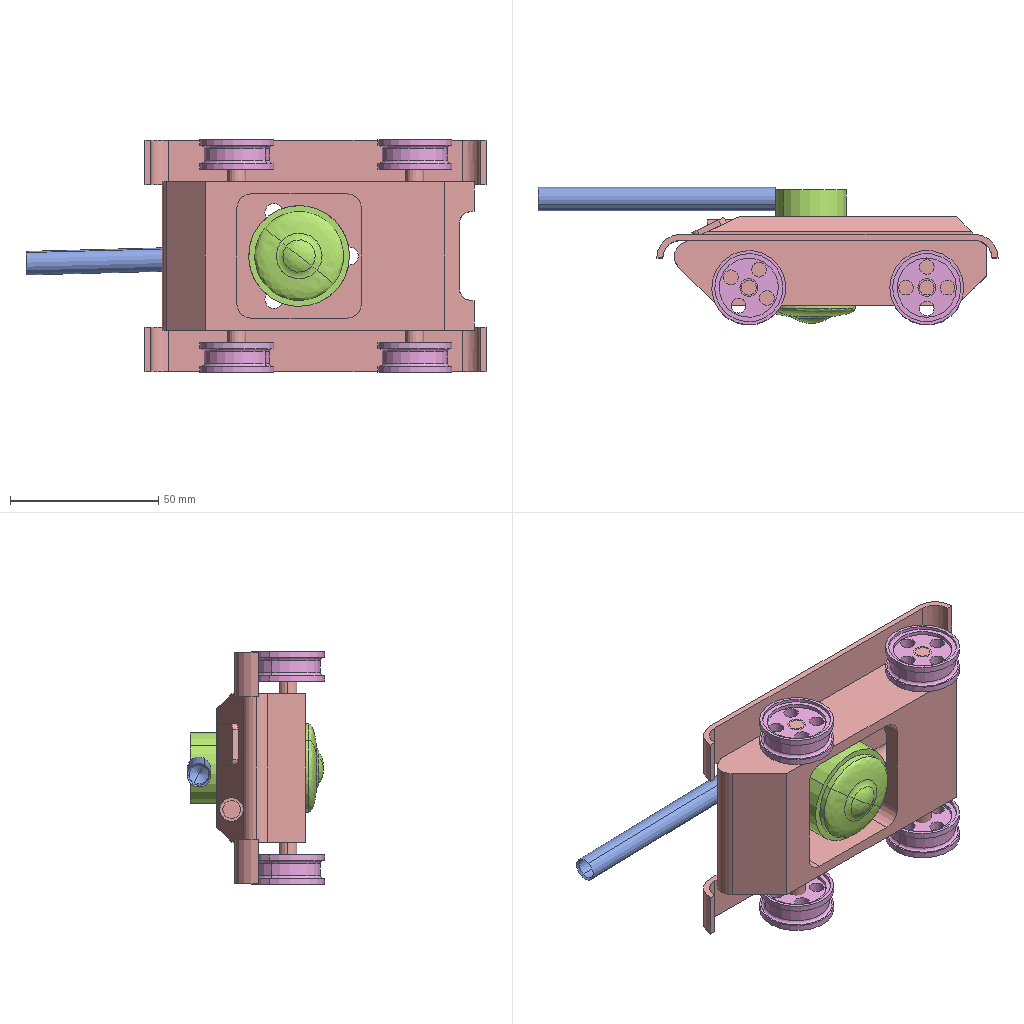Assembly | SolidWorks | 5 different items | 8 placed | box 155 x 46 x 78 mm
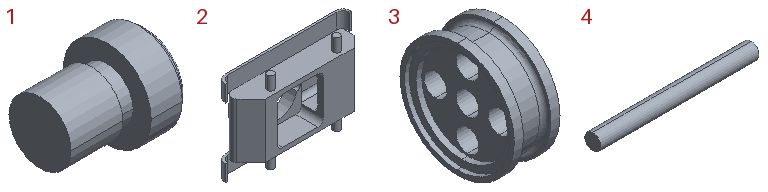Parts list (item | name | quantity | size | volume | features):
1 | - | x1 | 45 x 34 x 34 mm | 24801 mm3 | features Revolution 1
2 | - | x1 | 115 x 30 x 78 mm | 81134 mm3 | features ICE 9, Chamfer 1, Extrusion 1, MirrorPattern 1
3 | - | x4 | 10 x 25 x 25 mm | 2118 mm3 | features ICE 3, MirrorPattern 2, Revolution 1
4 | - | x1 | 79.975 x 8 x 8 mm | 3311 mm3 | features 3DProfileFeature 1, HoleWzd 1, Revolution 1
5 | Part7 | x1 | - | - | -
Mates (type | each side: item.copy, entity, surface, feature):
Concentric | 2.1 face cylinder Boss-Extrude4 | 3.1 face cylinder Cut-Extrude3
Coincident | 2.1 face plane Boss-Extrude4 | 3.1 face plane Cut-Extrude2
Concentric | 2.1 face cylinder Boss-Extrude4 | 3.2 face cylinder Cut-Extrude3
Coincident | 2.1 face plane Boss-Extrude4 | 3.2 face plane Cut-Extrude2
Tangent | 4.1 face plane Revolve1 | 1.1 face cylinder Revolve1